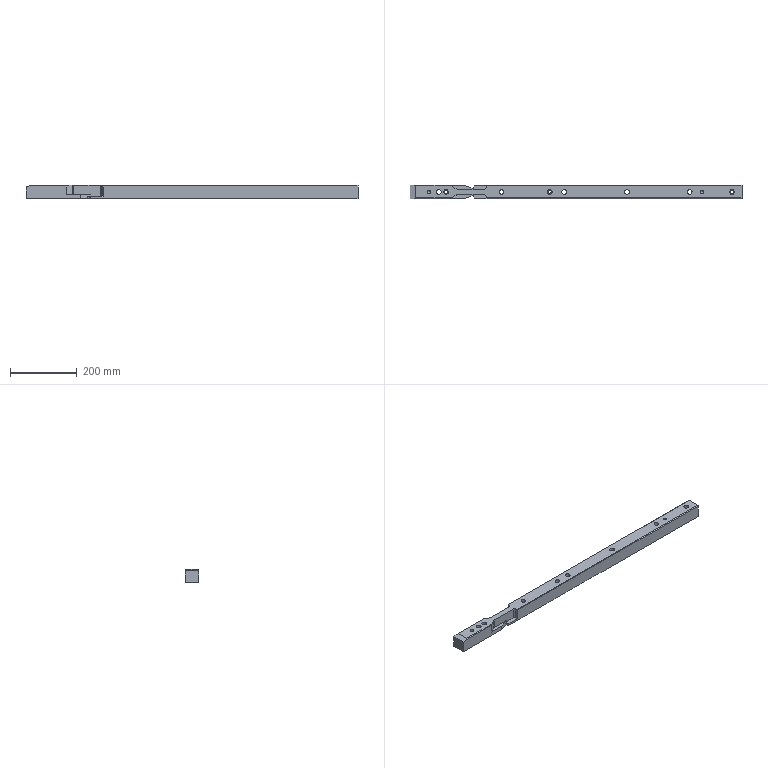Part | NX | features 22 2 | 1 solid | 68 faces | box 995 x 40 x 40 mm | volume 1449963 mm3 | plane 36 | cylinder 30 | cone 2 | commonest cylinder face diameters 14 x8 6 x6 10 x6 9 x3 25 x3 10.3 x2